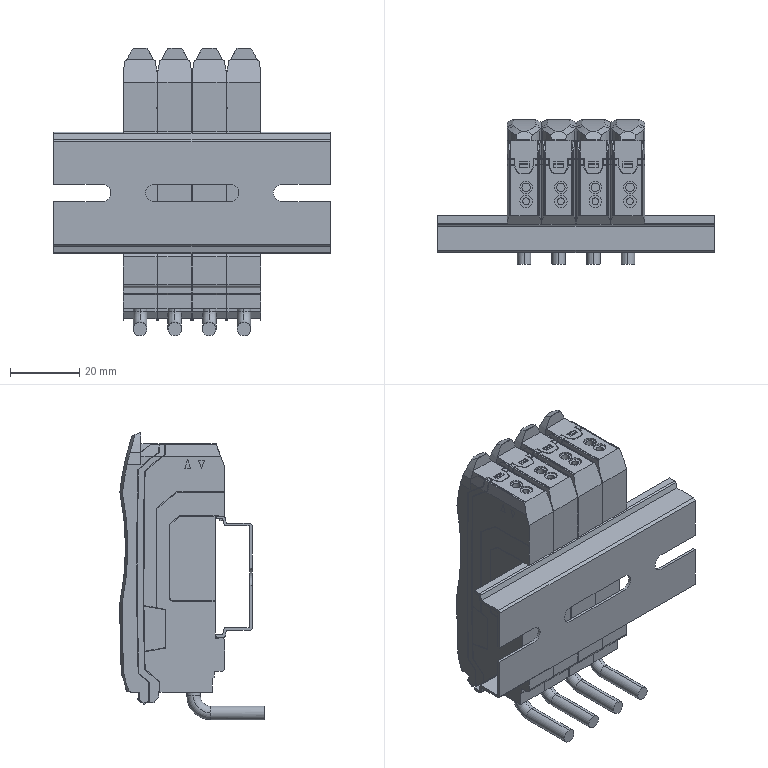Part | NX | 5 solids | 1294 faces | box 79.8 x 41.701 x 83.1 mm | volume 82231 mm3 | plane 926 | cylinder 288 | cone 36 | spline 32 | torus 12 | commonest cylinder face diameters 2 x36 1.66 x24 0.6 x16 3.628 x16 3.9 x16 1.601 x8